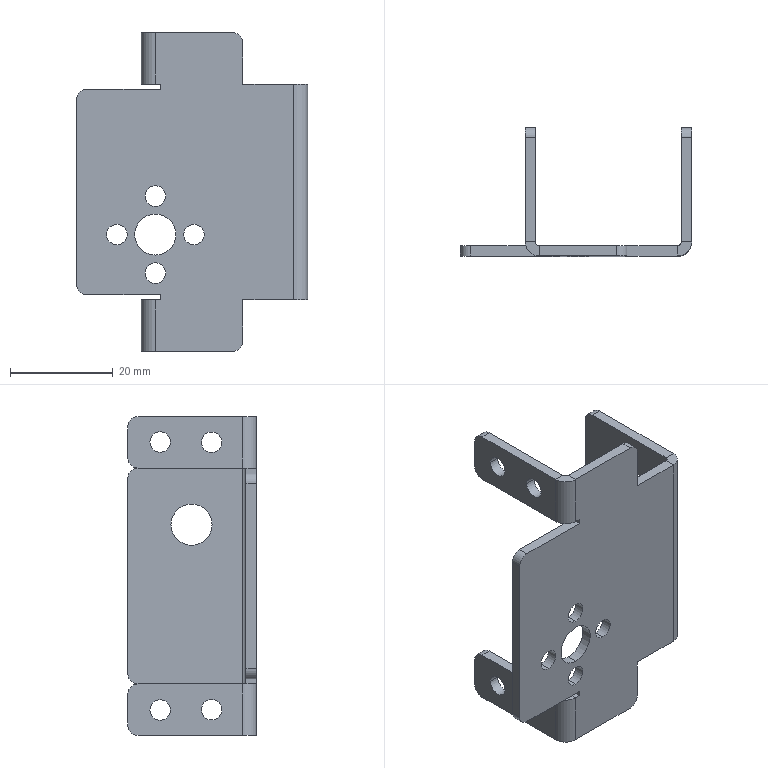Part | SolidWorks | features ICE 5, Fillet 3, EdgeFlange 2, SMBaseFlange 2, FlatPattern 1, MirrorPattern 1, SheetMetal 1 | 1 solid | 72 faces | box 45 x 25 x 62 mm | volume 6846 mm3 | cylinder 36 | plane 36 | commonest cylinder face diameters 4 x26 8 x4 1.473 x3 5.473 x3